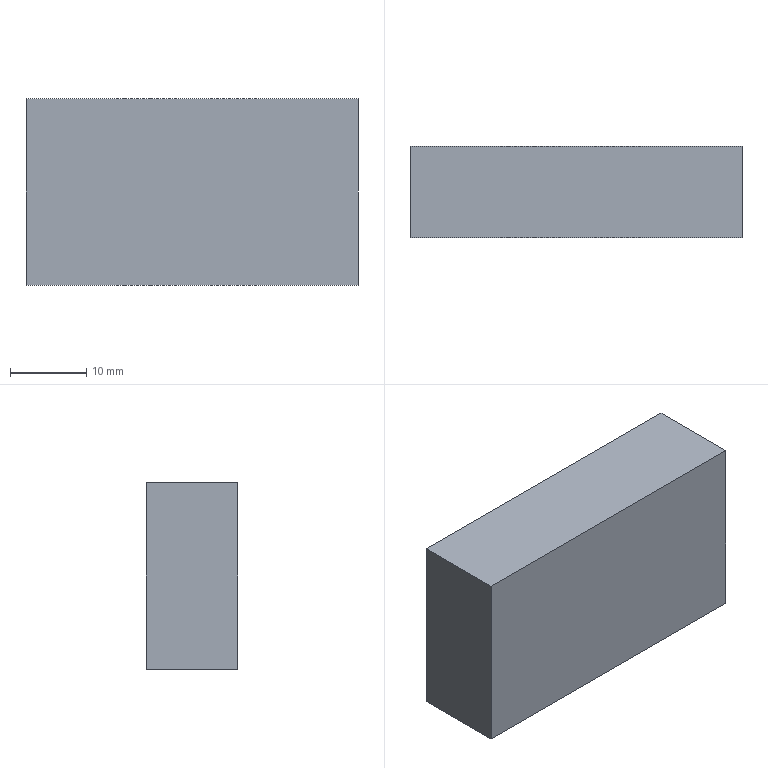Part | Creo | 1 solid | 6 faces | box 43.5 x 12 x 24.5 mm | volume 12789 mm3 | plane 6
STEP:
#1=CARTESIAN_POINT('',(0.,0.,0.));
#2=DIRECTION('',(0.,0.,1.));
#3=DIRECTION('',(1.,0.,0.));
#4=AXIS2_PLACEMENT_3D('',#1,#2,#3);
#5=CARTESIAN_POINT('',(-62.5,235.,-254.5));
#6=VERTEX_POINT('',#5);
#7=CARTESIAN_POINT('',(-19.,235.,-254.5));
#8=VERTEX_POINT('',#7);
#9=CARTESIAN_POINT('',(-62.5,235.,-254.5));
#10=DIRECTION('',(1.,0.,0.));
#11=VECTOR('',#10,43.5);
#12=LINE('',#9,#11);
#13=EDGE_CURVE('',#6,#8,#12,.T.);
#14=ORIENTED_EDGE('',*,*,#13,.F.);
#15=CARTESIAN_POINT('',(-62.5,247.,-254.5));
#16=VERTEX_POINT('',#15);
#17=CARTESIAN_POINT('',(-62.5,247.,-254.5));
#18=DIRECTION('',(0.,-1.,0.));
#19=VECTOR('',#18,12.);
#20=LINE('',#17,#19);
#21=EDGE_CURVE('',#16,#6,#20,.T.);
#22=ORIENTED_EDGE('',*,*,#21,.F.);
#23=CARTESIAN_POINT('',(-19.,247.,-254.5));
#24=VERTEX_POINT('',#23);
#25=CARTESIAN_POINT('',(-19.,247.,-254.5));
#26=DIRECTION('',(-1.,0.,0.));
#27=VECTOR('',#26,43.5);
#28=LINE('',#25,#27);
#29=EDGE_CURVE('',#24,#16,#28,.T.);
#30=ORIENTED_EDGE('',*,*,#29,.F.);
#31=CARTESIAN_POINT('',(-19.,235.,-254.5));
#32=DIRECTION('',(0.,1.,0.));
#33=VECTOR('',#32,12.);
#34=LINE('',#31,#33);
#35=EDGE_CURVE('',#8,#24,#34,.T.);
#36=ORIENTED_EDGE('',*,*,#35,.F.);
#37=EDGE_LOOP('',(#14,#22,#30,#36));
#38=FACE_OUTER_BOUND('',#37,.F.);
#39=CARTESIAN_POINT('',(-40.75,241.,-254.5));
#40=DIRECTION('',(0.,0.,1.));
#41=DIRECTION('',(1.,0.,0.));
#42=AXIS2_PLACEMENT_3D('',#39,#40,#41);
#43=PLANE('',#42);
#44=ADVANCED_FACE('',(#38),#43,.T.);
#45=CARTESIAN_POINT('',(-19.,235.,-279.));
#46=VERTEX_POINT('',#45);
#47=CARTESIAN_POINT('',(-19.,235.,-254.5));
#48=DIRECTION('',(0.,0.,-1.));
#49=VECTOR('',#48,24.5);
#50=LINE('',#47,#49);
#51=EDGE_CURVE('',#8,#46,#50,.T.);
#52=ORIENTED_EDGE('',*,*,#51,.T.);
#53=CARTESIAN_POINT('',(-62.5,235.,-279.));
#54=VERTEX_POINT('',#53);
#55=CARTESIAN_POINT('',(-19.,235.,-279.));
#56=DIRECTION('',(-1.,0.,0.));
#57=VECTOR('',#56,43.5);
#58=LINE('',#55,#57);
#59=EDGE_CURVE('',#46,#54,#58,.T.);
#60=ORIENTED_EDGE('',*,*,#59,.T.);
#61=CARTESIAN_POINT('',(-62.5,235.,-254.5));
#62=DIRECTION('',(0.,0.,-1.));
#63=VECTOR('',#62,24.5);
#64=LINE('',#61,#63);
#65=EDGE_CURVE('',#6,#54,#64,.T.);
#66=ORIENTED_EDGE('',*,*,#65,.F.);
#67=ORIENTED_EDGE('',*,*,#13,.T.);
#68=EDGE_LOOP('',(#52,#60,#66,#67));
#69=FACE_OUTER_BOUND('',#68,.F.);
#70=CARTESIAN_POINT('',(-40.75,235.,-279.));
#71=DIRECTION('',(0.,-1.,0.));
#72=DIRECTION('',(0.,0.,-1.));
#73=AXIS2_PLACEMENT_3D('',#70,#71,#72);
#74=PLANE('',#73);
#75=ADVANCED_FACE('',(#69),#74,.T.);
#76=CARTESIAN_POINT('',(-19.,247.,-279.));
#77=VERTEX_POINT('',#76);
#78=CARTESIAN_POINT('',(-19.,247.,-279.));
#79=DIRECTION('',(0.,-1.,0.));
#80=VECTOR('',#79,12.);
#81=LINE('',#78,#80);
#82=EDGE_CURVE('',#77,#46,#81,.T.);
#83=ORIENTED_EDGE('',*,*,#82,.T.);
#84=ORIENTED_EDGE('',*,*,#51,.F.);
#85=ORIENTED_EDGE('',*,*,#35,.T.);
#86=CARTESIAN_POINT('',(-19.,247.,-254.5));
#87=DIRECTION('',(0.,0.,-1.));
#88=VECTOR('',#87,24.5);
#89=LINE('',#86,#88);
#90=EDGE_CURVE('',#24,#77,#89,.T.);
#91=ORIENTED_EDGE('',*,*,#90,.T.);
#92=EDGE_LOOP('',(#83,#84,#85,#91));
#93=FACE_OUTER_BOUND('',#92,.F.);
#94=CARTESIAN_POINT('',(-19.,241.,-279.));
#95=DIRECTION('',(1.,0.,0.));
#96=DIRECTION('',(0.,0.,-1.));
#97=AXIS2_PLACEMENT_3D('',#94,#95,#96);
#98=PLANE('',#97);
#99=ADVANCED_FACE('',(#93),#98,.T.);
#100=ORIENTED_EDGE('',*,*,#82,.F.);
#101=CARTESIAN_POINT('',(-62.5,247.,-279.));
#102=VERTEX_POINT('',#101);
#103=CARTESIAN_POINT('',(-62.5,247.,-279.));
#104=DIRECTION('',(1.,0.,0.));
#105=VECTOR('',#104,43.5);
#106=LINE('',#103,#105);
#107=EDGE_CURVE('',#102,#77,#106,.T.);
#108=ORIENTED_EDGE('',*,*,#107,.F.);
#109=CARTESIAN_POINT('',(-62.5,235.,-279.));
#110=DIRECTION('',(0.,1.,0.));
#111=VECTOR('',#110,12.);
#112=LINE('',#109,#111);
#113=EDGE_CURVE('',#54,#102,#112,.T.);
#114=ORIENTED_EDGE('',*,*,#113,.F.);
#115=ORIENTED_EDGE('',*,*,#59,.F.);
#116=EDGE_LOOP('',(#100,#108,#114,#115));
#117=FACE_OUTER_BOUND('',#116,.F.);
#118=CARTESIAN_POINT('',(-40.75,241.,-279.));
#119=DIRECTION('',(0.,0.,-1.));
#120=DIRECTION('',(-1.,0.,0.));
#121=AXIS2_PLACEMENT_3D('',#118,#119,#120);
#122=PLANE('',#121);
#123=ADVANCED_FACE('',(#117),#122,.T.);
#124=CARTESIAN_POINT('',(-62.5,247.,-254.5));
#125=DIRECTION('',(0.,0.,-1.));
#126=VECTOR('',#125,24.5);
#127=LINE('',#124,#126);
#128=EDGE_CURVE('',#16,#102,#127,.T.);
#129=ORIENTED_EDGE('',*,*,#128,.T.);
#130=ORIENTED_EDGE('',*,*,#107,.T.);
#131=ORIENTED_EDGE('',*,*,#90,.F.);
#132=ORIENTED_EDGE('',*,*,#29,.T.);
#133=EDGE_LOOP('',(#129,#130,#131,#132));
#134=FACE_OUTER_BOUND('',#133,.F.);
#135=CARTESIAN_POINT('',(-40.75,247.,-279.));
#136=DIRECTION('',(0.,1.,0.));
#137=DIRECTION('',(0.,0.,1.));
#138=AXIS2_PLACEMENT_3D('',#135,#136,#137);
#139=PLANE('',#138);
#140=ADVANCED_FACE('',(#134),#139,.T.);
#141=ORIENTED_EDGE('',*,*,#65,.T.);
#142=ORIENTED_EDGE('',*,*,#113,.T.);
#143=ORIENTED_EDGE('',*,*,#128,.F.);
#144=ORIENTED_EDGE('',*,*,#21,.T.);
#145=EDGE_LOOP('',(#141,#142,#143,#144));
#146=FACE_OUTER_BOUND('',#145,.F.);
#147=CARTESIAN_POINT('',(-62.5,241.,-279.));
#148=DIRECTION('',(-1.,0.,0.));
#149=DIRECTION('',(0.,0.,1.));
#150=AXIS2_PLACEMENT_3D('',#147,#148,#149);
#151=PLANE('',#150);
#152=ADVANCED_FACE('',(#146),#151,.T.);
#153=CLOSED_SHELL('',(#44,#75,#99,#123,#140,#152));
#154=MANIFOLD_SOLID_BREP('',#153);
#155=(LENGTH_UNIT()NAMED_UNIT(*)SI_UNIT(.MILLI.,.METRE.));
#156=UNCERTAINTY_MEASURE_WITH_UNIT(LENGTH_MEASURE(0.005134),#155,'','');
#157=(NAMED_UNIT(*)PLANE_ANGLE_UNIT()SI_UNIT($,.RADIAN.));
#158=PLANE_ANGLE_MEASURE_WITH_UNIT(PLANE_ANGLE_MEASURE(0.01745),#157);
#159=(CONVERSION_BASED_UNIT('DEGREE',#158)NAMED_UNIT(*)PLANE_ANGLE_UNIT());
#160=(NAMED_UNIT(*)SI_UNIT($,.STERADIAN.)SOLID_ANGLE_UNIT());
#161=(GEOMETRIC_REPRESENTATION_CONTEXT(3)GLOBAL_UNCERTAINTY_ASSIGNED_CONTEXT((#156))GLOBAL_UNIT_ASSIGNED_CONTEXT((#155,#159,#160))REPRESENTATION_CONTEXT('',''));
#162=ADVANCED_BREP_SHAPE_REPRESENTATION('',(#4,#154),#161);